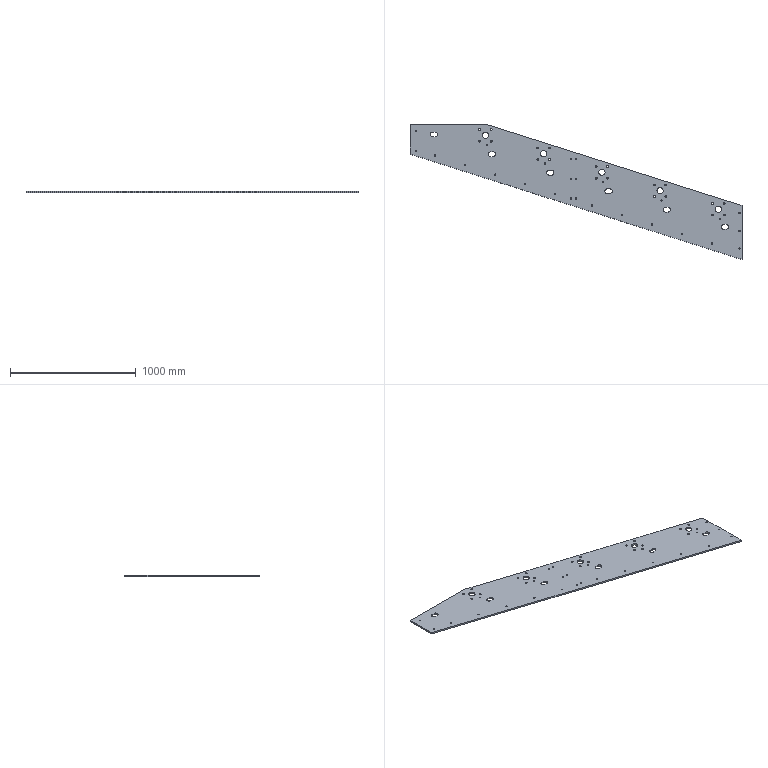Part | SolidWorks | features Cut 7, LPattern 5, ICE 2, Extrusion 1, SurfCut 1 | 1 solid | 139 faces | box 2640 x 1075 x 12 mm | volume 12600247 mm3 | cylinder 120 | plane 19 | commonest cylinder face diameters 10 x52 15 x40 38 x18 50 x10